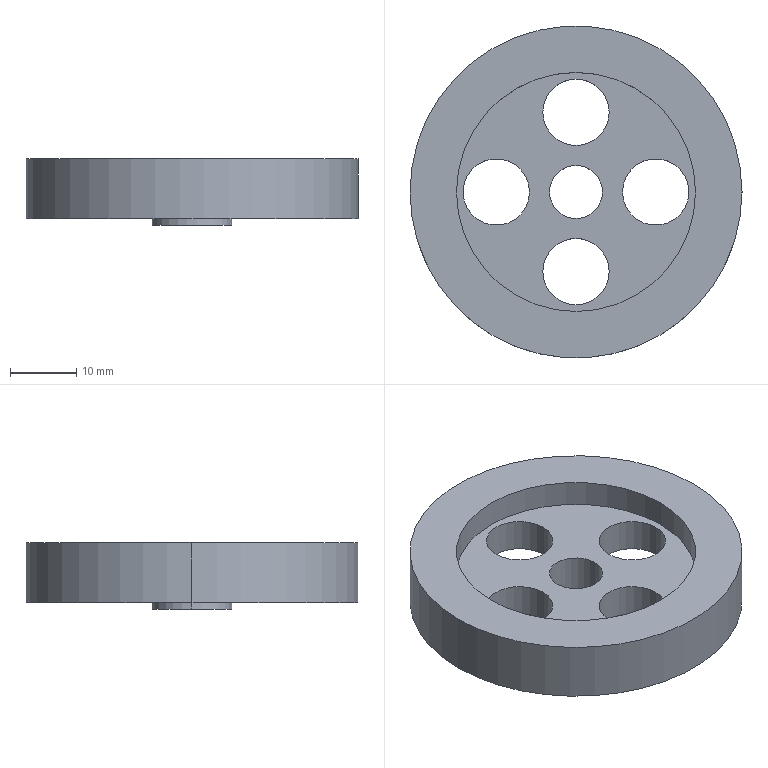Part | SolidWorks | features ICE 4, Extrusion 1 | 1 solid | 20 faces | box 50 x 50 x 10 mm | volume 11841 mm3 | cylinder 16 | plane 4 | commonest cylinder face diameters 10 x8 8 x2 12 x2 36 x2 50 x2
STEP:
#1=CARTESIAN_POINT('',(-6.,0.,-1.));
#2=VERTEX_POINT('',#1);
#3=CARTESIAN_POINT('',(6.,0.,-1.));
#4=VERTEX_POINT('',#3);
#5=CARTESIAN_POINT('',(0.,0.,-1.));
#6=DIRECTION('',(0.,0.,-1.));
#7=DIRECTION('',(-1.,0.,0.));
#8=AXIS2_PLACEMENT_3D('',#5,#6,#7);
#9=CIRCLE('',#8,6.);
#10=EDGE_CURVE('',#2,#4,#9,.T.);
#11=ORIENTED_EDGE('',*,*,#10,.F.);
#12=CARTESIAN_POINT('',(-6.,0.,0.));
#13=VERTEX_POINT('',#12);
#14=CARTESIAN_POINT('',(-6.,0.,-1.));
#15=DIRECTION('',(0.,0.,1.));
#16=VECTOR('',#15,1000.);
#17=LINE('',#14,#16);
#18=EDGE_CURVE('',#2,#13,#17,.T.);
#19=ORIENTED_EDGE('',*,*,#18,.T.);
#20=CARTESIAN_POINT('',(6.,0.,0.));
#21=VERTEX_POINT('',#20);
#22=CARTESIAN_POINT('',(0.,0.,0.));
#23=DIRECTION('',(0.,0.,-1.));
#24=DIRECTION('',(1.,0.,0.));
#25=AXIS2_PLACEMENT_3D('',#22,#23,#24);
#26=CIRCLE('',#25,6.);
#27=EDGE_CURVE('',#13,#21,#26,.T.);
#28=ORIENTED_EDGE('',*,*,#27,.T.);
#29=CARTESIAN_POINT('',(6.,0.,-1.));
#30=DIRECTION('',(0.,0.,1.));
#31=VECTOR('',#30,1000.);
#32=LINE('',#29,#31);
#33=EDGE_CURVE('',#4,#21,#32,.T.);
#34=ORIENTED_EDGE('',*,*,#33,.F.);
#35=EDGE_LOOP('',(#11,#19,#28,#34));
#36=FACE_OUTER_BOUND('',#35,.T.);
#37=CARTESIAN_POINT('',(0.,0.,-1.));
#38=DIRECTION('',(0.,0.,1.));
#39=DIRECTION('',(1.,0.,0.));
#40=AXIS2_PLACEMENT_3D('',#37,#38,#39);
#41=CYLINDRICAL_SURFACE('',#40,6.);
#42=ADVANCED_FACE('',(#36),#41,.T.);
#43=CARTESIAN_POINT('',(4.,0.,-1.));
#44=VERTEX_POINT('',#43);
#45=CARTESIAN_POINT('',(-4.,0.,-1.));
#46=VERTEX_POINT('',#45);
#47=CARTESIAN_POINT('',(0.,0.,-1.));
#48=DIRECTION('',(0.,0.,-1.));
#49=DIRECTION('',(-1.,0.,0.));
#50=AXIS2_PLACEMENT_3D('',#47,#48,#49);
#51=CIRCLE('',#50,4.);
#52=EDGE_CURVE('',#44,#46,#51,.T.);
#53=ORIENTED_EDGE('',*,*,#52,.T.);
#54=CARTESIAN_POINT('',(-4.,0.,5.));
#55=VERTEX_POINT('',#54);
#56=CARTESIAN_POINT('',(-4.,0.,0.));
#57=DIRECTION('',(0.,0.,1.));
#58=VECTOR('',#57,1000.);
#59=LINE('',#56,#58);
#60=EDGE_CURVE('',#46,#55,#59,.T.);
#61=ORIENTED_EDGE('',*,*,#60,.T.);
#62=CARTESIAN_POINT('',(4.,0.,5.));
#63=VERTEX_POINT('',#62);
#64=CARTESIAN_POINT('',(0.,0.,5.));
#65=DIRECTION('',(0.,0.,1.));
#66=DIRECTION('',(1.,0.,0.));
#67=AXIS2_PLACEMENT_3D('',#64,#65,#66);
#68=CIRCLE('',#67,4.);
#69=EDGE_CURVE('',#55,#63,#68,.T.);
#70=ORIENTED_EDGE('',*,*,#69,.T.);
#71=CARTESIAN_POINT('',(4.,0.,0.));
#72=DIRECTION('',(0.,0.,1.));
#73=VECTOR('',#72,1000.);
#74=LINE('',#71,#73);
#75=EDGE_CURVE('',#44,#63,#74,.T.);
#76=ORIENTED_EDGE('',*,*,#75,.F.);
#77=EDGE_LOOP('',(#53,#61,#70,#76));
#78=FACE_OUTER_BOUND('',#77,.T.);
#79=CARTESIAN_POINT('',(0.,0.,0.));
#80=DIRECTION('',(0.,0.,1.));
#81=DIRECTION('',(1.,0.,0.));
#82=AXIS2_PLACEMENT_3D('',#79,#80,#81);
#83=CYLINDRICAL_SURFACE('',#82,4.);
#84=ADVANCED_FACE('',(#78),#83,.F.);
#85=CARTESIAN_POINT('',(-5.,12.,0.));
#86=VERTEX_POINT('',#85);
#87=CARTESIAN_POINT('',(5.,12.,0.));
#88=VERTEX_POINT('',#87);
#89=CARTESIAN_POINT('',(0.,12.,0.));
#90=DIRECTION('',(0.,0.,1.));
#91=DIRECTION('',(1.,0.,0.));
#92=AXIS2_PLACEMENT_3D('',#89,#90,#91);
#93=CIRCLE('',#92,5.);
#94=EDGE_CURVE('',#86,#88,#93,.T.);
#95=ORIENTED_EDGE('',*,*,#94,.F.);
#96=CARTESIAN_POINT('',(-5.,12.,5.));
#97=VERTEX_POINT('',#96);
#98=CARTESIAN_POINT('',(-5.,12.,0.));
#99=DIRECTION('',(0.,0.,1.));
#100=VECTOR('',#99,1000.);
#101=LINE('',#98,#100);
#102=EDGE_CURVE('',#86,#97,#101,.T.);
#103=ORIENTED_EDGE('',*,*,#102,.T.);
#104=CARTESIAN_POINT('',(5.,12.,5.));
#105=VERTEX_POINT('',#104);
#106=CARTESIAN_POINT('',(0.,12.,5.));
#107=DIRECTION('',(0.,0.,1.));
#108=DIRECTION('',(1.,0.,0.));
#109=AXIS2_PLACEMENT_3D('',#106,#107,#108);
#110=CIRCLE('',#109,5.);
#111=EDGE_CURVE('',#97,#105,#110,.T.);
#112=ORIENTED_EDGE('',*,*,#111,.T.);
#113=CARTESIAN_POINT('',(5.,12.,0.));
#114=DIRECTION('',(0.,0.,1.));
#115=VECTOR('',#114,1000.);
#116=LINE('',#113,#115);
#117=EDGE_CURVE('',#88,#105,#116,.T.);
#118=ORIENTED_EDGE('',*,*,#117,.F.);
#119=EDGE_LOOP('',(#95,#103,#112,#118));
#120=FACE_OUTER_BOUND('',#119,.T.);
#121=CARTESIAN_POINT('',(0.,12.,0.));
#122=DIRECTION('',(0.,0.,1.));
#123=DIRECTION('',(1.,0.,0.));
#124=AXIS2_PLACEMENT_3D('',#121,#122,#123);
#125=CYLINDRICAL_SURFACE('',#124,5.);
#126=ADVANCED_FACE('',(#120),#125,.F.);
#127=CARTESIAN_POINT('',(7.,0.,0.));
#128=VERTEX_POINT('',#127);
#129=CARTESIAN_POINT('',(17.,0.,0.));
#130=VERTEX_POINT('',#129);
#131=CARTESIAN_POINT('',(12.,0.,0.));
#132=DIRECTION('',(0.,0.,1.));
#133=DIRECTION('',(1.,0.,0.));
#134=AXIS2_PLACEMENT_3D('',#131,#132,#133);
#135=CIRCLE('',#134,5.);
#136=EDGE_CURVE('',#128,#130,#135,.T.);
#137=ORIENTED_EDGE('',*,*,#136,.F.);
#138=CARTESIAN_POINT('',(7.,0.,5.));
#139=VERTEX_POINT('',#138);
#140=CARTESIAN_POINT('',(7.,0.,0.));
#141=DIRECTION('',(0.,0.,1.));
#142=VECTOR('',#141,1000.);
#143=LINE('',#140,#142);
#144=EDGE_CURVE('',#128,#139,#143,.T.);
#145=ORIENTED_EDGE('',*,*,#144,.T.);
#146=CARTESIAN_POINT('',(17.,0.,5.));
#147=VERTEX_POINT('',#146);
#148=CARTESIAN_POINT('',(12.,0.,5.));
#149=DIRECTION('',(0.,0.,1.));
#150=DIRECTION('',(1.,0.,0.));
#151=AXIS2_PLACEMENT_3D('',#148,#149,#150);
#152=CIRCLE('',#151,5.);
#153=EDGE_CURVE('',#139,#147,#152,.T.);
#154=ORIENTED_EDGE('',*,*,#153,.T.);
#155=CARTESIAN_POINT('',(17.,0.,0.));
#156=DIRECTION('',(0.,0.,1.));
#157=VECTOR('',#156,1000.);
#158=LINE('',#155,#157);
#159=EDGE_CURVE('',#130,#147,#158,.T.);
#160=ORIENTED_EDGE('',*,*,#159,.F.);
#161=EDGE_LOOP('',(#137,#145,#154,#160));
#162=FACE_OUTER_BOUND('',#161,.T.);
#163=CARTESIAN_POINT('',(12.,0.,0.));
#164=DIRECTION('',(0.,0.,1.));
#165=DIRECTION('',(1.,0.,0.));
#166=AXIS2_PLACEMENT_3D('',#163,#164,#165);
#167=CYLINDRICAL_SURFACE('',#166,5.);
#168=ADVANCED_FACE('',(#162),#167,.F.);
#169=CARTESIAN_POINT('',(-5.,-12.,0.));
#170=VERTEX_POINT('',#169);
#171=CARTESIAN_POINT('',(5.,-12.,0.));
#172=VERTEX_POINT('',#171);
#173=CARTESIAN_POINT('',(0.,-12.,0.));
#174=DIRECTION('',(0.,0.,1.));
#175=DIRECTION('',(1.,0.,0.));
#176=AXIS2_PLACEMENT_3D('',#173,#174,#175);
#177=CIRCLE('',#176,5.);
#178=EDGE_CURVE('',#170,#172,#177,.T.);
#179=ORIENTED_EDGE('',*,*,#178,.F.);
#180=CARTESIAN_POINT('',(-5.,-12.,5.));
#181=VERTEX_POINT('',#180);
#182=CARTESIAN_POINT('',(-5.,-12.,0.));
#183=DIRECTION('',(0.,0.,1.));
#184=VECTOR('',#183,1000.);
#185=LINE('',#182,#184);
#186=EDGE_CURVE('',#170,#181,#185,.T.);
#187=ORIENTED_EDGE('',*,*,#186,.T.);
#188=CARTESIAN_POINT('',(5.,-12.,5.));
#189=VERTEX_POINT('',#188);
#190=CARTESIAN_POINT('',(0.,-12.,5.));
#191=DIRECTION('',(0.,0.,1.));
#192=DIRECTION('',(1.,0.,0.));
#193=AXIS2_PLACEMENT_3D('',#190,#191,#192);
#194=CIRCLE('',#193,5.);
#195=EDGE_CURVE('',#181,#189,#194,.T.);
#196=ORIENTED_EDGE('',*,*,#195,.T.);
#197=CARTESIAN_POINT('',(5.,-12.,0.));
#198=DIRECTION('',(0.,0.,1.));
#199=VECTOR('',#198,1000.);
#200=LINE('',#197,#199);
#201=EDGE_CURVE('',#172,#189,#200,.T.);
#202=ORIENTED_EDGE('',*,*,#201,.F.);
#203=EDGE_LOOP('',(#179,#187,#196,#202));
#204=FACE_OUTER_BOUND('',#203,.T.);
#205=CARTESIAN_POINT('',(0.,-12.,0.));
#206=DIRECTION('',(0.,0.,1.));
#207=DIRECTION('',(1.,0.,0.));
#208=AXIS2_PLACEMENT_3D('',#205,#206,#207);
#209=CYLINDRICAL_SURFACE('',#208,5.);
#210=ADVANCED_FACE('',(#204),#209,.F.);
#211=CARTESIAN_POINT('',(-17.,0.,0.));
#212=VERTEX_POINT('',#211);
#213=CARTESIAN_POINT('',(-7.,0.,0.));
#214=VERTEX_POINT('',#213);
#215=CARTESIAN_POINT('',(-12.,0.,0.));
#216=DIRECTION('',(0.,0.,1.));
#217=DIRECTION('',(1.,0.,0.));
#218=AXIS2_PLACEMENT_3D('',#215,#216,#217);
#219=CIRCLE('',#218,5.);
#220=EDGE_CURVE('',#212,#214,#219,.T.);
#221=ORIENTED_EDGE('',*,*,#220,.F.);
#222=CARTESIAN_POINT('',(-17.,0.,5.));
#223=VERTEX_POINT('',#222);
#224=CARTESIAN_POINT('',(-17.,0.,0.));
#225=DIRECTION('',(0.,0.,1.));
#226=VECTOR('',#225,1000.);
#227=LINE('',#224,#226);
#228=EDGE_CURVE('',#212,#223,#227,.T.);
#229=ORIENTED_EDGE('',*,*,#228,.T.);
#230=CARTESIAN_POINT('',(-7.,0.,5.));
#231=VERTEX_POINT('',#230);
#232=CARTESIAN_POINT('',(-12.,0.,5.));
#233=DIRECTION('',(0.,0.,1.));
#234=DIRECTION('',(1.,0.,0.));
#235=AXIS2_PLACEMENT_3D('',#232,#233,#234);
#236=CIRCLE('',#235,5.);
#237=EDGE_CURVE('',#223,#231,#236,.T.);
#238=ORIENTED_EDGE('',*,*,#237,.T.);
#239=CARTESIAN_POINT('',(-7.,0.,0.));
#240=DIRECTION('',(0.,0.,1.));
#241=VECTOR('',#240,1000.);
#242=LINE('',#239,#241);
#243=EDGE_CURVE('',#214,#231,#242,.T.);
#244=ORIENTED_EDGE('',*,*,#243,.F.);
#245=EDGE_LOOP('',(#221,#229,#238,#244));
#246=FACE_OUTER_BOUND('',#245,.T.);
#247=CARTESIAN_POINT('',(-12.,0.,0.));
#248=DIRECTION('',(0.,0.,1.));
#249=DIRECTION('',(1.,0.,0.));
#250=AXIS2_PLACEMENT_3D('',#247,#248,#249);
#251=CYLINDRICAL_SURFACE('',#250,5.);
#252=ADVANCED_FACE('',(#246),#251,.F.);
#253=CARTESIAN_POINT('',(-18.,0.,5.));
#254=VERTEX_POINT('',#253);
#255=CARTESIAN_POINT('',(18.,0.,5.));
#256=VERTEX_POINT('',#255);
#257=CARTESIAN_POINT('',(0.,0.,5.));
#258=DIRECTION('',(0.,0.,1.));
#259=DIRECTION('',(1.,0.,0.));
#260=AXIS2_PLACEMENT_3D('',#257,#258,#259);
#261=CIRCLE('',#260,18.);
#262=EDGE_CURVE('',#254,#256,#261,.T.);
#263=ORIENTED_EDGE('',*,*,#262,.F.);
#264=CARTESIAN_POINT('',(-18.,0.,9.));
#265=VERTEX_POINT('',#264);
#266=CARTESIAN_POINT('',(-18.,0.,5.));
#267=DIRECTION('',(0.,0.,1.));
#268=VECTOR('',#267,1000.);
#269=LINE('',#266,#268);
#270=EDGE_CURVE('',#254,#265,#269,.T.);
#271=ORIENTED_EDGE('',*,*,#270,.T.);
#272=CARTESIAN_POINT('',(18.,0.,9.));
#273=VERTEX_POINT('',#272);
#274=CARTESIAN_POINT('',(0.,0.,9.));
#275=DIRECTION('',(0.,0.,1.));
#276=DIRECTION('',(1.,0.,0.));
#277=AXIS2_PLACEMENT_3D('',#274,#275,#276);
#278=CIRCLE('',#277,18.);
#279=EDGE_CURVE('',#265,#273,#278,.T.);
#280=ORIENTED_EDGE('',*,*,#279,.T.);
#281=CARTESIAN_POINT('',(18.,0.,5.));
#282=DIRECTION('',(0.,0.,1.));
#283=VECTOR('',#282,1000.);
#284=LINE('',#281,#283);
#285=EDGE_CURVE('',#256,#273,#284,.T.);
#286=ORIENTED_EDGE('',*,*,#285,.F.);
#287=EDGE_LOOP('',(#263,#271,#280,#286));
#288=FACE_OUTER_BOUND('',#287,.T.);
#289=CARTESIAN_POINT('',(0.,0.,5.));
#290=DIRECTION('',(0.,0.,1.));
#291=DIRECTION('',(1.,0.,0.));
#292=AXIS2_PLACEMENT_3D('',#289,#290,#291);
#293=CYLINDRICAL_SURFACE('',#292,18.);
#294=ADVANCED_FACE('',(#288),#293,.F.);
#295=CARTESIAN_POINT('',(25.,0.,9.));
#296=VERTEX_POINT('',#295);
#297=CARTESIAN_POINT('',(-25.,0.,9.));
#298=VERTEX_POINT('',#297);
#299=CARTESIAN_POINT('',(0.,0.,9.));
#300=DIRECTION('',(0.,0.,1.));
#301=DIRECTION('',(1.,0.,0.));
#302=AXIS2_PLACEMENT_3D('',#299,#300,#301);
#303=CIRCLE('',#302,25.);
#304=EDGE_CURVE('',#296,#298,#303,.T.);
#305=ORIENTED_EDGE('',*,*,#304,.F.);
#306=CARTESIAN_POINT('',(25.,0.,0.));
#307=VERTEX_POINT('',#306);
#308=CARTESIAN_POINT('',(25.,0.,9.));
#309=DIRECTION('',(0.,0.,-1.));
#310=VECTOR('',#309,1000.);
#311=LINE('',#308,#310);
#312=EDGE_CURVE('',#296,#307,#311,.T.);
#313=ORIENTED_EDGE('',*,*,#312,.T.);
#314=CARTESIAN_POINT('',(-25.,0.,0.));
#315=VERTEX_POINT('',#314);
#316=CARTESIAN_POINT('',(0.,0.,0.));
#317=DIRECTION('',(0.,0.,1.));
#318=DIRECTION('',(1.,0.,0.));
#319=AXIS2_PLACEMENT_3D('',#316,#317,#318);
#320=CIRCLE('',#319,25.);
#321=EDGE_CURVE('',#307,#315,#320,.T.);
#322=ORIENTED_EDGE('',*,*,#321,.T.);
#323=CARTESIAN_POINT('',(-25.,0.,9.));
#324=DIRECTION('',(0.,0.,-1.));
#325=VECTOR('',#324,1000.);
#326=LINE('',#323,#325);
#327=EDGE_CURVE('',#298,#315,#326,.T.);
#328=ORIENTED_EDGE('',*,*,#327,.F.);
#329=EDGE_LOOP('',(#305,#313,#322,#328));
#330=FACE_OUTER_BOUND('',#329,.T.);
#331=CARTESIAN_POINT('',(0.,0.,9.));
#332=DIRECTION('',(0.,0.,-1.));
#333=DIRECTION('',(-1.,0.,0.));
#334=AXIS2_PLACEMENT_3D('',#331,#332,#333);
#335=CYLINDRICAL_SURFACE('',#334,25.);
#336=ADVANCED_FACE('',(#330),#335,.T.);
#337=CARTESIAN_POINT('',(0.,0.,0.));
#338=DIRECTION('',(0.,0.,1.));
#339=DIRECTION('',(1.,0.,0.));
#340=AXIS2_PLACEMENT_3D('',#337,#338,#339);
#341=CIRCLE('',#340,25.);
#342=EDGE_CURVE('',#315,#307,#341,.T.);
#343=ORIENTED_EDGE('',*,*,#342,.F.);
#344=ORIENTED_EDGE('',*,*,#321,.F.);
#345=EDGE_LOOP('',(#343,#344));
#346=FACE_OUTER_BOUND('',#345,.T.);
#347=CARTESIAN_POINT('',(-12.,0.,0.));
#348=DIRECTION('',(0.,0.,1.));
#349=DIRECTION('',(1.,0.,0.));
#350=AXIS2_PLACEMENT_3D('',#347,#348,#349);
#351=CIRCLE('',#350,5.);
#352=EDGE_CURVE('',#214,#212,#351,.T.);
#353=ORIENTED_EDGE('',*,*,#352,.T.);
#354=ORIENTED_EDGE('',*,*,#220,.T.);
#355=EDGE_LOOP('',(#353,#354));
#356=FACE_BOUND('',#355,.T.);
#357=CARTESIAN_POINT('',(0.,-12.,0.));
#358=DIRECTION('',(0.,0.,1.));
#359=DIRECTION('',(1.,0.,0.));
#360=AXIS2_PLACEMENT_3D('',#357,#358,#359);
#361=CIRCLE('',#360,5.);
#362=EDGE_CURVE('',#172,#170,#361,.T.);
#363=ORIENTED_EDGE('',*,*,#362,.T.);
#364=ORIENTED_EDGE('',*,*,#178,.T.);
#365=EDGE_LOOP('',(#363,#364));
#366=FACE_BOUND('',#365,.T.);
#367=CARTESIAN_POINT('',(12.,0.,0.));
#368=DIRECTION('',(0.,0.,1.));
#369=DIRECTION('',(1.,0.,0.));
#370=AXIS2_PLACEMENT_3D('',#367,#368,#369);
#371=CIRCLE('',#370,5.);
#372=EDGE_CURVE('',#130,#128,#371,.T.);
#373=ORIENTED_EDGE('',*,*,#372,.T.);
#374=ORIENTED_EDGE('',*,*,#136,.T.);
#375=EDGE_LOOP('',(#373,#374));
#376=FACE_BOUND('',#375,.T.);
#377=CARTESIAN_POINT('',(0.,12.,0.));
#378=DIRECTION('',(0.,0.,1.));
#379=DIRECTION('',(1.,0.,0.));
#380=AXIS2_PLACEMENT_3D('',#377,#378,#379);
#381=CIRCLE('',#380,5.);
#382=EDGE_CURVE('',#88,#86,#381,.T.);
#383=ORIENTED_EDGE('',*,*,#382,.T.);
#384=ORIENTED_EDGE('',*,*,#94,.T.);
#385=EDGE_LOOP('',(#383,#384));
#386=FACE_BOUND('',#385,.T.);
#387=CARTESIAN_POINT('',(0.,0.,0.));
#388=DIRECTION('',(0.,0.,-1.));
#389=DIRECTION('',(1.,0.,0.));
#390=AXIS2_PLACEMENT_3D('',#387,#388,#389);
#391=CIRCLE('',#390,6.);
#392=EDGE_CURVE('',#21,#13,#391,.T.);
#393=ORIENTED_EDGE('',*,*,#392,.F.);
#394=ORIENTED_EDGE('',*,*,#27,.F.);
#395=EDGE_LOOP('',(#393,#394));
#396=FACE_BOUND('',#395,.T.);
#397=CARTESIAN_POINT('',(0.,0.,0.));
#398=DIRECTION('',(0.,0.,1.));
#399=DIRECTION('',(1.,0.,0.));
#400=AXIS2_PLACEMENT_3D('',#397,#398,#399);
#401=PLANE('',#400);
#402=ADVANCED_FACE('',(#346,#356,#366,#376,#386,#396),#401,.F.);
#403=ORIENTED_EDGE('',*,*,#312,.F.);
#404=CARTESIAN_POINT('',(0.,0.,9.));
#405=DIRECTION('',(0.,0.,1.));
#406=DIRECTION('',(1.,0.,0.));
#407=AXIS2_PLACEMENT_3D('',#404,#405,#406);
#408=CIRCLE('',#407,25.);
#409=EDGE_CURVE('',#298,#296,#408,.T.);
#410=ORIENTED_EDGE('',*,*,#409,.F.);
#411=ORIENTED_EDGE('',*,*,#327,.T.);
#412=ORIENTED_EDGE('',*,*,#342,.T.);
#413=EDGE_LOOP('',(#403,#410,#411,#412));
#414=FACE_OUTER_BOUND('',#413,.T.);
#415=CARTESIAN_POINT('',(0.,0.,9.));
#416=DIRECTION('',(0.,0.,-1.));
#417=DIRECTION('',(-1.,0.,0.));
#418=AXIS2_PLACEMENT_3D('',#415,#416,#417);
#419=CYLINDRICAL_SURFACE('',#418,25.);
#420=ADVANCED_FACE('',(#414),#419,.T.);
#421=CARTESIAN_POINT('',(0.,0.,9.));
#422=DIRECTION('',(0.,0.,1.));
#423=DIRECTION('',(1.,0.,0.));
#424=AXIS2_PLACEMENT_3D('',#421,#422,#423);
#425=CIRCLE('',#424,18.);
#426=EDGE_CURVE('',#273,#265,#425,.T.);
#427=ORIENTED_EDGE('',*,*,#426,.F.);
#428=ORIENTED_EDGE('',*,*,#279,.F.);
#429=EDGE_LOOP('',(#427,#428));
#430=FACE_BOUND('',#429,.T.);
#431=ORIENTED_EDGE('',*,*,#409,.T.);
#432=ORIENTED_EDGE('',*,*,#304,.T.);
#433=EDGE_LOOP('',(#431,#432));
#434=FACE_OUTER_BOUND('',#433,.T.);
#435=CARTESIAN_POINT('',(0.,0.,9.));
#436=DIRECTION('',(0.,0.,1.));
#437=DIRECTION('',(1.,0.,0.));
#438=AXIS2_PLACEMENT_3D('',#435,#436,#437);
#439=PLANE('',#438);
#440=ADVANCED_FACE('',(#430,#434),#439,.T.);
#441=ORIENTED_EDGE('',*,*,#270,.F.);
#442=CARTESIAN_POINT('',(0.,0.,5.));
#443=DIRECTION('',(0.,0.,1.));
#444=DIRECTION('',(1.,0.,0.));
#445=AXIS2_PLACEMENT_3D('',#442,#443,#444);
#446=CIRCLE('',#445,18.);
#447=EDGE_CURVE('',#256,#254,#446,.T.);
#448=ORIENTED_EDGE('',*,*,#447,.F.);
#449=ORIENTED_EDGE('',*,*,#285,.T.);
#450=ORIENTED_EDGE('',*,*,#426,.T.);
#451=EDGE_LOOP('',(#441,#448,#449,#450));
#452=FACE_OUTER_BOUND('',#451,.T.);
#453=CARTESIAN_POINT('',(0.,0.,5.));
#454=DIRECTION('',(0.,0.,1.));
#455=DIRECTION('',(1.,0.,0.));
#456=AXIS2_PLACEMENT_3D('',#453,#454,#455);
#457=CYLINDRICAL_SURFACE('',#456,18.);
#458=ADVANCED_FACE('',(#452),#457,.F.);
#459=CARTESIAN_POINT('',(0.,0.,5.));
#460=DIRECTION('',(0.,0.,1.));
#461=DIRECTION('',(1.,0.,0.));
#462=AXIS2_PLACEMENT_3D('',#459,#460,#461);
#463=CIRCLE('',#462,4.);
#464=EDGE_CURVE('',#63,#55,#463,.T.);
#465=ORIENTED_EDGE('',*,*,#464,.F.);
#466=ORIENTED_EDGE('',*,*,#69,.F.);
#467=EDGE_LOOP('',(#465,#466));
#468=FACE_BOUND('',#467,.T.);
#469=CARTESIAN_POINT('',(0.,12.,5.));
#470=DIRECTION('',(0.,0.,1.));
#471=DIRECTION('',(1.,0.,0.));
#472=AXIS2_PLACEMENT_3D('',#469,#470,#471);
#473=CIRCLE('',#472,5.);
#474=EDGE_CURVE('',#105,#97,#473,.T.);
#475=ORIENTED_EDGE('',*,*,#474,.F.);
#476=ORIENTED_EDGE('',*,*,#111,.F.);
#477=EDGE_LOOP('',(#475,#476));
#478=FACE_BOUND('',#477,.T.);
#479=CARTESIAN_POINT('',(12.,0.,5.));
#480=DIRECTION('',(0.,0.,1.));
#481=DIRECTION('',(1.,0.,0.));
#482=AXIS2_PLACEMENT_3D('',#479,#480,#481);
#483=CIRCLE('',#482,5.);
#484=EDGE_CURVE('',#147,#139,#483,.T.);
#485=ORIENTED_EDGE('',*,*,#484,.F.);
#486=ORIENTED_EDGE('',*,*,#153,.F.);
#487=EDGE_LOOP('',(#485,#486));
#488=FACE_BOUND('',#487,.T.);
#489=CARTESIAN_POINT('',(0.,-12.,5.));
#490=DIRECTION('',(0.,0.,1.));
#491=DIRECTION('',(1.,0.,0.));
#492=AXIS2_PLACEMENT_3D('',#489,#490,#491);
#493=CIRCLE('',#492,5.);
#494=EDGE_CURVE('',#189,#181,#493,.T.);
#495=ORIENTED_EDGE('',*,*,#494,.F.);
#496=ORIENTED_EDGE('',*,*,#195,.F.);
#497=EDGE_LOOP('',(#495,#496));
#498=FACE_BOUND('',#497,.T.);
#499=CARTESIAN_POINT('',(-12.,0.,5.));
#500=DIRECTION('',(0.,0.,1.));
#501=DIRECTION('',(1.,0.,0.));
#502=AXIS2_PLACEMENT_3D('',#499,#500,#501);
#503=CIRCLE('',#502,5.);
#504=EDGE_CURVE('',#231,#223,#503,.T.);
#505=ORIENTED_EDGE('',*,*,#504,.F.);
#506=ORIENTED_EDGE('',*,*,#237,.F.);
#507=EDGE_LOOP('',(#505,#506));
#508=FACE_BOUND('',#507,.T.);
#509=ORIENTED_EDGE('',*,*,#447,.T.);
#510=ORIENTED_EDGE('',*,*,#262,.T.);
#511=EDGE_LOOP('',(#509,#510));
#512=FACE_OUTER_BOUND('',#511,.T.);
#513=CARTESIAN_POINT('',(0.,0.,5.));
#514=DIRECTION('',(0.,0.,1.));
#515=DIRECTION('',(1.,0.,0.));
#516=AXIS2_PLACEMENT_3D('',#513,#514,#515);
#517=PLANE('',#516);
#518=ADVANCED_FACE('',(#468,#478,#488,#498,#508,#512),#517,.T.);
#519=ORIENTED_EDGE('',*,*,#228,.F.);
#520=ORIENTED_EDGE('',*,*,#352,.F.);
#521=ORIENTED_EDGE('',*,*,#243,.T.);
#522=ORIENTED_EDGE('',*,*,#504,.T.);
#523=EDGE_LOOP('',(#519,#520,#521,#522));
#524=FACE_OUTER_BOUND('',#523,.T.);
#525=CARTESIAN_POINT('',(-12.,0.,0.));
#526=DIRECTION('',(0.,0.,1.));
#527=DIRECTION('',(1.,0.,0.));
#528=AXIS2_PLACEMENT_3D('',#525,#526,#527);
#529=CYLINDRICAL_SURFACE('',#528,5.);
#530=ADVANCED_FACE('',(#524),#529,.F.);
#531=ORIENTED_EDGE('',*,*,#186,.F.);
#532=ORIENTED_EDGE('',*,*,#362,.F.);
#533=ORIENTED_EDGE('',*,*,#201,.T.);
#534=ORIENTED_EDGE('',*,*,#494,.T.);
#535=EDGE_LOOP('',(#531,#532,#533,#534));
#536=FACE_OUTER_BOUND('',#535,.T.);
#537=CARTESIAN_POINT('',(0.,-12.,0.));
#538=DIRECTION('',(0.,0.,1.));
#539=DIRECTION('',(1.,0.,0.));
#540=AXIS2_PLACEMENT_3D('',#537,#538,#539);
#541=CYLINDRICAL_SURFACE('',#540,5.);
#542=ADVANCED_FACE('',(#536),#541,.F.);
#543=ORIENTED_EDGE('',*,*,#144,.F.);
#544=ORIENTED_EDGE('',*,*,#372,.F.);
#545=ORIENTED_EDGE('',*,*,#159,.T.);
#546=ORIENTED_EDGE('',*,*,#484,.T.);
#547=EDGE_LOOP('',(#543,#544,#545,#546));
#548=FACE_OUTER_BOUND('',#547,.T.);
#549=CARTESIAN_POINT('',(12.,0.,0.));
#550=DIRECTION('',(0.,0.,1.));
#551=DIRECTION('',(1.,0.,0.));
#552=AXIS2_PLACEMENT_3D('',#549,#550,#551);
#553=CYLINDRICAL_SURFACE('',#552,5.);
#554=ADVANCED_FACE('',(#548),#553,.F.);
#555=ORIENTED_EDGE('',*,*,#102,.F.);
#556=ORIENTED_EDGE('',*,*,#382,.F.);
#557=ORIENTED_EDGE('',*,*,#117,.T.);
#558=ORIENTED_EDGE('',*,*,#474,.T.);
#559=EDGE_LOOP('',(#555,#556,#557,#558));
#560=FACE_OUTER_BOUND('',#559,.T.);
#561=CARTESIAN_POINT('',(0.,12.,0.));
#562=DIRECTION('',(0.,0.,1.));
#563=DIRECTION('',(1.,0.,0.));
#564=AXIS2_PLACEMENT_3D('',#561,#562,#563);
#565=CYLINDRICAL_SURFACE('',#564,5.);
#566=ADVANCED_FACE('',(#560),#565,.F.);
#567=ORIENTED_EDGE('',*,*,#60,.F.);
#568=CARTESIAN_POINT('',(0.,0.,-1.));
#569=DIRECTION('',(0.,0.,-1.));
#570=DIRECTION('',(-1.,0.,0.));
#571=AXIS2_PLACEMENT_3D('',#568,#569,#570);
#572=CIRCLE('',#571,4.);
#573=EDGE_CURVE('',#46,#44,#572,.T.);
#574=ORIENTED_EDGE('',*,*,#573,.T.);
#575=ORIENTED_EDGE('',*,*,#75,.T.);
#576=ORIENTED_EDGE('',*,*,#464,.T.);
#577=EDGE_LOOP('',(#567,#574,#575,#576));
#578=FACE_OUTER_BOUND('',#577,.T.);
#579=CARTESIAN_POINT('',(0.,0.,0.));
#580=DIRECTION('',(0.,0.,1.));
#581=DIRECTION('',(1.,0.,0.));
#582=AXIS2_PLACEMENT_3D('',#579,#580,#581);
#583=CYLINDRICAL_SURFACE('',#582,4.);
#584=ADVANCED_FACE('',(#578),#583,.F.);
#585=CARTESIAN_POINT('',(0.,0.,-1.));
#586=DIRECTION('',(0.,0.,-1.));
#587=DIRECTION('',(-1.,0.,0.));
#588=AXIS2_PLACEMENT_3D('',#585,#586,#587);
#589=CIRCLE('',#588,6.);
#590=EDGE_CURVE('',#4,#2,#589,.T.);
#591=ORIENTED_EDGE('',*,*,#590,.T.);
#592=ORIENTED_EDGE('',*,*,#10,.T.);
#593=EDGE_LOOP('',(#591,#592));
#594=FACE_OUTER_BOUND('',#593,.T.);
#595=ORIENTED_EDGE('',*,*,#52,.F.);
#596=ORIENTED_EDGE('',*,*,#573,.F.);
#597=EDGE_LOOP('',(#595,#596));
#598=FACE_BOUND('',#597,.T.);
#599=CARTESIAN_POINT('',(0.,0.,-1.));
#600=DIRECTION('',(0.,0.,-1.));
#601=DIRECTION('',(-1.,0.,0.));
#602=AXIS2_PLACEMENT_3D('',#599,#600,#601);
#603=PLANE('',#602);
#604=ADVANCED_FACE('',(#594,#598),#603,.T.);
#605=ORIENTED_EDGE('',*,*,#18,.F.);
#606=ORIENTED_EDGE('',*,*,#590,.F.);
#607=ORIENTED_EDGE('',*,*,#33,.T.);
#608=ORIENTED_EDGE('',*,*,#392,.T.);
#609=EDGE_LOOP('',(#605,#606,#607,#608));
#610=FACE_OUTER_BOUND('',#609,.T.);
#611=CARTESIAN_POINT('',(0.,0.,-1.));
#612=DIRECTION('',(0.,0.,1.));
#613=DIRECTION('',(1.,0.,0.));
#614=AXIS2_PLACEMENT_3D('',#611,#612,#613);
#615=CYLINDRICAL_SURFACE('',#614,6.);
#616=ADVANCED_FACE('',(#610),#615,.T.);
#617=CLOSED_SHELL('',(#42,#84,#126,#168,#210,#252,#294,#336,#402,#420,#440,#458,#518,#530,#542,#554,#566,#584,#604,#616));
#618=MANIFOLD_SOLID_BREP('',#617);
#619=CARTESIAN_POINT('',(0.,0.,0.));
#620=DIRECTION('',(0.,0.,1.));
#621=DIRECTION('',(1.,0.,0.));
#622=AXIS2_PLACEMENT_3D('',#619,#620,#621);
#623=(LENGTH_UNIT()NAMED_UNIT(*)SI_UNIT(.MILLI.,.METRE.));
#624=UNCERTAINTY_MEASURE_WITH_UNIT(LENGTH_MEASURE(0.00001),#623,'','');
#625=(NAMED_UNIT(*)PLANE_ANGLE_UNIT()SI_UNIT($,.RADIAN.));
#626=(NAMED_UNIT(*)SI_UNIT($,.STERADIAN.)SOLID_ANGLE_UNIT());
#627=(GEOMETRIC_REPRESENTATION_CONTEXT(3)GLOBAL_UNCERTAINTY_ASSIGNED_CONTEXT((#624))GLOBAL_UNIT_ASSIGNED_CONTEXT((#623,#625,#626))REPRESENTATION_CONTEXT('',''));
#628=ADVANCED_BREP_SHAPE_REPRESENTATION('',(#618,#622),#627);